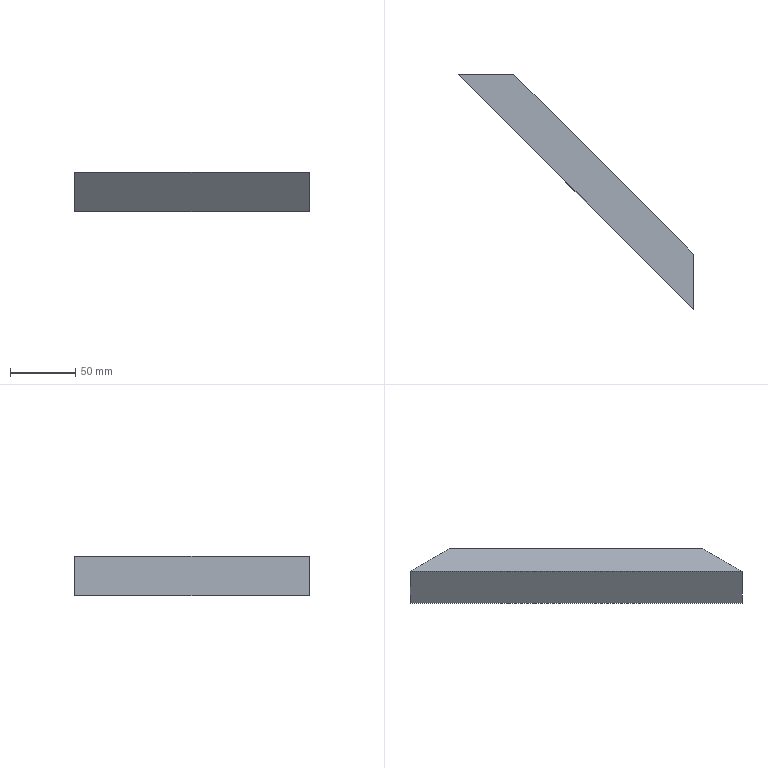Part | NX | features solid 2 | 1 solid | 10 faces | box 180 x 180 x 30 mm | volume 50301 mm3 | plane 10
STEP:
#1=CARTESIAN_POINT('',(212.426,-330.,-60.));
#2=VERTEX_POINT('',#1);
#3=CARTESIAN_POINT('',(170.,-330.,-60.));
#4=VERTEX_POINT('',#3);
#5=CARTESIAN_POINT('',(320.,-330.,-60.));
#6=DIRECTION('',(-1.,0.,0.));
#7=VECTOR('',#6,1000.);
#8=LINE('',#5,#7);
#9=EDGE_CURVE('',#2,#4,#8,.T.);
#10=ORIENTED_EDGE('',*,*,#9,.T.);
#11=CARTESIAN_POINT('',(170.,-330.,-30.));
#12=VERTEX_POINT('',#11);
#13=CARTESIAN_POINT('',(170.,-330.,-30.));
#14=DIRECTION('',(0.,0.,-1.));
#15=VECTOR('',#14,1000.);
#16=LINE('',#13,#15);
#17=EDGE_CURVE('',#12,#4,#16,.T.);
#18=ORIENTED_EDGE('',*,*,#17,.F.);
#19=CARTESIAN_POINT('',(212.426,-330.,-30.));
#20=VERTEX_POINT('',#19);
#21=CARTESIAN_POINT('',(320.,-330.,-30.));
#22=DIRECTION('',(-1.,0.,0.));
#23=VECTOR('',#22,1000.);
#24=LINE('',#21,#23);
#25=EDGE_CURVE('',#20,#12,#24,.T.);
#26=ORIENTED_EDGE('',*,*,#25,.F.);
#27=CARTESIAN_POINT('',(212.426,-330.,-30.));
#28=DIRECTION('',(0.,0.,-1.));
#29=VECTOR('',#28,1000.);
#30=LINE('',#27,#29);
#31=EDGE_CURVE('',#20,#2,#30,.T.);
#32=ORIENTED_EDGE('',*,*,#31,.T.);
#33=EDGE_LOOP('',(#10,#18,#26,#32));
#34=FACE_BOUND('',#33,.T.);
#35=CARTESIAN_POINT('',(209.598,-330.,-32.));
#36=VERTEX_POINT('',#35);
#37=CARTESIAN_POINT('',(209.598,-330.,-58.));
#38=VERTEX_POINT('',#37);
#39=CARTESIAN_POINT('',(209.598,-330.,-30.));
#40=DIRECTION('',(0.,0.,-1.));
#41=VECTOR('',#40,1000.);
#42=LINE('',#39,#41);
#43=EDGE_CURVE('',#36,#38,#42,.T.);
#44=ORIENTED_EDGE('',*,*,#43,.F.);
#45=CARTESIAN_POINT('',(172.828,-330.,-32.));
#46=VERTEX_POINT('',#45);
#47=CARTESIAN_POINT('',(320.,-330.,-32.));
#48=DIRECTION('',(-1.,0.,0.));
#49=VECTOR('',#48,1000.);
#50=LINE('',#47,#49);
#51=EDGE_CURVE('',#36,#46,#50,.T.);
#52=ORIENTED_EDGE('',*,*,#51,.T.);
#53=CARTESIAN_POINT('',(172.828,-330.,-58.));
#54=VERTEX_POINT('',#53);
#55=CARTESIAN_POINT('',(172.828,-330.,-30.));
#56=DIRECTION('',(0.,0.,-1.));
#57=VECTOR('',#56,1000.);
#58=LINE('',#55,#57);
#59=EDGE_CURVE('',#46,#54,#58,.T.);
#60=ORIENTED_EDGE('',*,*,#59,.T.);
#61=CARTESIAN_POINT('',(320.,-330.,-58.));
#62=DIRECTION('',(-1.,0.,0.));
#63=VECTOR('',#62,1000.);
#64=LINE('',#61,#63);
#65=EDGE_CURVE('',#38,#54,#64,.T.);
#66=ORIENTED_EDGE('',*,*,#65,.F.);
#67=EDGE_LOOP('',(#44,#52,#60,#66));
#68=FACE_BOUND('',#67,.T.);
#69=CARTESIAN_POINT('',(320.,-330.,-30.));
#70=DIRECTION('',(0.,1.,0.));
#71=DIRECTION('',(0.,0.,1.));
#72=AXIS2_PLACEMENT_3D('',#69,#70,#71);
#73=PLANE('',#72);
#74=ADVANCED_FACE('',(#34,#68),#73,.T.);
#75=CARTESIAN_POINT('',(350.,-510.,-60.));
#76=VERTEX_POINT('',#75);
#77=CARTESIAN_POINT('',(350.,-467.574,-60.));
#78=VERTEX_POINT('',#77);
#79=CARTESIAN_POINT('',(350.,-402.5,-60.));
#80=DIRECTION('',(0.,1.,0.));
#81=VECTOR('',#80,1000.);
#82=LINE('',#79,#81);
#83=EDGE_CURVE('',#76,#78,#82,.T.);
#84=ORIENTED_EDGE('',*,*,#83,.T.);
#85=CARTESIAN_POINT('',(350.,-467.574,-30.));
#86=VERTEX_POINT('',#85);
#87=CARTESIAN_POINT('',(350.,-467.574,-30.));
#88=DIRECTION('',(0.,0.,-1.));
#89=VECTOR('',#88,1000.);
#90=LINE('',#87,#89);
#91=EDGE_CURVE('',#86,#78,#90,.T.);
#92=ORIENTED_EDGE('',*,*,#91,.F.);
#93=CARTESIAN_POINT('',(350.,-510.,-30.));
#94=VERTEX_POINT('',#93);
#95=CARTESIAN_POINT('',(350.,-402.5,-30.));
#96=DIRECTION('',(0.,1.,0.));
#97=VECTOR('',#96,1000.);
#98=LINE('',#95,#97);
#99=EDGE_CURVE('',#94,#86,#98,.T.);
#100=ORIENTED_EDGE('',*,*,#99,.F.);
#101=CARTESIAN_POINT('',(350.,-510.,-30.));
#102=DIRECTION('',(0.,0.,-1.));
#103=VECTOR('',#102,1000.);
#104=LINE('',#101,#103);
#105=EDGE_CURVE('',#94,#76,#104,.T.);
#106=ORIENTED_EDGE('',*,*,#105,.T.);
#107=EDGE_LOOP('',(#84,#92,#100,#106));
#108=FACE_BOUND('',#107,.T.);
#109=CARTESIAN_POINT('',(350.,-507.172,-32.));
#110=VERTEX_POINT('',#109);
#111=CARTESIAN_POINT('',(350.,-507.172,-58.));
#112=VERTEX_POINT('',#111);
#113=CARTESIAN_POINT('',(350.,-507.172,-30.));
#114=DIRECTION('',(0.,0.,-1.));
#115=VECTOR('',#114,1000.);
#116=LINE('',#113,#115);
#117=EDGE_CURVE('',#110,#112,#116,.T.);
#118=ORIENTED_EDGE('',*,*,#117,.F.);
#119=CARTESIAN_POINT('',(350.,-470.402,-32.));
#120=VERTEX_POINT('',#119);
#121=CARTESIAN_POINT('',(350.,-402.5,-32.));
#122=DIRECTION('',(0.,1.,0.));
#123=VECTOR('',#122,1000.);
#124=LINE('',#121,#123);
#125=EDGE_CURVE('',#110,#120,#124,.T.);
#126=ORIENTED_EDGE('',*,*,#125,.T.);
#127=CARTESIAN_POINT('',(350.,-470.402,-58.));
#128=VERTEX_POINT('',#127);
#129=CARTESIAN_POINT('',(350.,-470.402,-30.));
#130=DIRECTION('',(0.,0.,-1.));
#131=VECTOR('',#130,1000.);
#132=LINE('',#129,#131);
#133=EDGE_CURVE('',#120,#128,#132,.T.);
#134=ORIENTED_EDGE('',*,*,#133,.T.);
#135=CARTESIAN_POINT('',(350.,-402.5,-58.));
#136=DIRECTION('',(0.,1.,0.));
#137=VECTOR('',#136,1000.);
#138=LINE('',#135,#137);
#139=EDGE_CURVE('',#112,#128,#138,.T.);
#140=ORIENTED_EDGE('',*,*,#139,.F.);
#141=EDGE_LOOP('',(#118,#126,#134,#140));
#142=FACE_BOUND('',#141,.T.);
#143=CARTESIAN_POINT('',(350.,-620.,-30.));
#144=DIRECTION('',(1.,0.,0.));
#145=DIRECTION('',(0.,0.,1.));
#146=AXIS2_PLACEMENT_3D('',#143,#144,#145);
#147=PLANE('',#146);
#148=ADVANCED_FACE('',(#108,#142),#147,.T.);
#149=CARTESIAN_POINT('',(212.426,-330.,-60.));
#150=DIRECTION('',(0.7071,-0.7071,0.));
#151=VECTOR('',#150,1000.);
#152=LINE('',#149,#151);
#153=EDGE_CURVE('',#2,#78,#152,.T.);
#154=ORIENTED_EDGE('',*,*,#153,.F.);
#155=ORIENTED_EDGE('',*,*,#31,.F.);
#156=CARTESIAN_POINT('',(212.426,-330.,-30.));
#157=DIRECTION('',(0.7071,-0.7071,0.));
#158=VECTOR('',#157,1000.);
#159=LINE('',#156,#158);
#160=EDGE_CURVE('',#20,#86,#159,.T.);
#161=ORIENTED_EDGE('',*,*,#160,.T.);
#162=ORIENTED_EDGE('',*,*,#91,.T.);
#163=EDGE_LOOP('',(#154,#155,#161,#162));
#164=FACE_BOUND('',#163,.T.);
#165=CARTESIAN_POINT('',(212.426,-330.,-30.));
#166=DIRECTION('',(-0.7071,-0.7071,0.));
#167=DIRECTION('',(-0.7071,0.7071,0.));
#168=AXIS2_PLACEMENT_3D('',#165,#166,#167);
#169=PLANE('',#168);
#170=ADVANCED_FACE('',(#164),#169,.F.);
#171=CARTESIAN_POINT('',(170.,-330.,-60.));
#172=DIRECTION('',(0.7071,-0.7071,0.));
#173=VECTOR('',#172,1000.);
#174=LINE('',#171,#173);
#175=EDGE_CURVE('',#4,#76,#174,.T.);
#176=ORIENTED_EDGE('',*,*,#175,.T.);
#177=ORIENTED_EDGE('',*,*,#105,.F.);
#178=CARTESIAN_POINT('',(170.,-330.,-30.));
#179=DIRECTION('',(0.7071,-0.7071,0.));
#180=VECTOR('',#179,1000.);
#181=LINE('',#178,#180);
#182=EDGE_CURVE('',#12,#94,#181,.T.);
#183=ORIENTED_EDGE('',*,*,#182,.F.);
#184=ORIENTED_EDGE('',*,*,#17,.T.);
#185=EDGE_LOOP('',(#176,#177,#183,#184));
#186=FACE_BOUND('',#185,.T.);
#187=CARTESIAN_POINT('',(170.,-330.,-30.));
#188=DIRECTION('',(-0.7071,-0.7071,0.));
#189=DIRECTION('',(-0.7071,0.7071,0.));
#190=AXIS2_PLACEMENT_3D('',#187,#188,#189);
#191=PLANE('',#190);
#192=ADVANCED_FACE('',(#186),#191,.T.);
#193=ORIENTED_EDGE('',*,*,#25,.T.);
#194=ORIENTED_EDGE('',*,*,#182,.T.);
#195=ORIENTED_EDGE('',*,*,#99,.T.);
#196=ORIENTED_EDGE('',*,*,#160,.F.);
#197=EDGE_LOOP('',(#193,#194,#195,#196));
#198=FACE_BOUND('',#197,.T.);
#199=CARTESIAN_POINT('',(255.607,-402.5,-30.));
#200=DIRECTION('',(0.,0.,1.));
#201=DIRECTION('',(-1.,0.,0.));
#202=AXIS2_PLACEMENT_3D('',#199,#200,#201);
#203=PLANE('',#202);
#204=ADVANCED_FACE('',(#198),#203,.T.);
#205=ORIENTED_EDGE('',*,*,#9,.F.);
#206=ORIENTED_EDGE('',*,*,#153,.T.);
#207=ORIENTED_EDGE('',*,*,#83,.F.);
#208=ORIENTED_EDGE('',*,*,#175,.F.);
#209=EDGE_LOOP('',(#205,#206,#207,#208));
#210=FACE_BOUND('',#209,.T.);
#211=CARTESIAN_POINT('',(255.607,-402.5,-60.));
#212=DIRECTION('',(0.,0.,1.));
#213=DIRECTION('',(-1.,0.,0.));
#214=AXIS2_PLACEMENT_3D('',#211,#212,#213);
#215=PLANE('',#214);
#216=ADVANCED_FACE('',(#210),#215,.F.);
#217=CARTESIAN_POINT('',(211.012,-331.414,-58.));
#218=DIRECTION('',(0.7071,-0.7071,0.));
#219=VECTOR('',#218,1000.);
#220=LINE('',#217,#219);
#221=EDGE_CURVE('',#38,#128,#220,.T.);
#222=ORIENTED_EDGE('',*,*,#221,.T.);
#223=ORIENTED_EDGE('',*,*,#133,.F.);
#224=CARTESIAN_POINT('',(211.012,-331.414,-32.));
#225=DIRECTION('',(0.7071,-0.7071,0.));
#226=VECTOR('',#225,1000.);
#227=LINE('',#224,#226);
#228=EDGE_CURVE('',#36,#120,#227,.T.);
#229=ORIENTED_EDGE('',*,*,#228,.F.);
#230=ORIENTED_EDGE('',*,*,#43,.T.);
#231=EDGE_LOOP('',(#222,#223,#229,#230));
#232=FACE_BOUND('',#231,.T.);
#233=CARTESIAN_POINT('',(211.012,-331.414,-30.));
#234=DIRECTION('',(-0.7071,-0.7071,0.));
#235=DIRECTION('',(-0.7071,0.7071,0.));
#236=AXIS2_PLACEMENT_3D('',#233,#234,#235);
#237=PLANE('',#236);
#238=ADVANCED_FACE('',(#232),#237,.T.);
#239=CARTESIAN_POINT('',(171.414,-328.586,-58.));
#240=DIRECTION('',(0.7071,-0.7071,0.));
#241=VECTOR('',#240,1000.);
#242=LINE('',#239,#241);
#243=EDGE_CURVE('',#54,#112,#242,.T.);
#244=ORIENTED_EDGE('',*,*,#243,.F.);
#245=ORIENTED_EDGE('',*,*,#59,.F.);
#246=CARTESIAN_POINT('',(171.414,-328.586,-32.));
#247=DIRECTION('',(0.7071,-0.7071,0.));
#248=VECTOR('',#247,1000.);
#249=LINE('',#246,#248);
#250=EDGE_CURVE('',#46,#110,#249,.T.);
#251=ORIENTED_EDGE('',*,*,#250,.T.);
#252=ORIENTED_EDGE('',*,*,#117,.T.);
#253=EDGE_LOOP('',(#244,#245,#251,#252));
#254=FACE_BOUND('',#253,.T.);
#255=CARTESIAN_POINT('',(171.414,-328.586,-30.));
#256=DIRECTION('',(-0.7071,-0.7071,0.));
#257=DIRECTION('',(-0.7071,0.7071,0.));
#258=AXIS2_PLACEMENT_3D('',#255,#256,#257);
#259=PLANE('',#258);
#260=ADVANCED_FACE('',(#254),#259,.F.);
#261=ORIENTED_EDGE('',*,*,#51,.F.);
#262=ORIENTED_EDGE('',*,*,#228,.T.);
#263=ORIENTED_EDGE('',*,*,#125,.F.);
#264=ORIENTED_EDGE('',*,*,#250,.F.);
#265=EDGE_LOOP('',(#261,#262,#263,#264));
#266=FACE_BOUND('',#265,.T.);
#267=CARTESIAN_POINT('',(255.607,-402.5,-32.));
#268=DIRECTION('',(0.,0.,1.));
#269=DIRECTION('',(-1.,0.,0.));
#270=AXIS2_PLACEMENT_3D('',#267,#268,#269);
#271=PLANE('',#270);
#272=ADVANCED_FACE('',(#266),#271,.F.);
#273=ORIENTED_EDGE('',*,*,#65,.T.);
#274=ORIENTED_EDGE('',*,*,#243,.T.);
#275=ORIENTED_EDGE('',*,*,#139,.T.);
#276=ORIENTED_EDGE('',*,*,#221,.F.);
#277=EDGE_LOOP('',(#273,#274,#275,#276));
#278=FACE_BOUND('',#277,.T.);
#279=CARTESIAN_POINT('',(255.607,-402.5,-58.));
#280=DIRECTION('',(0.,0.,1.));
#281=DIRECTION('',(-1.,0.,0.));
#282=AXIS2_PLACEMENT_3D('',#279,#280,#281);
#283=PLANE('',#282);
#284=ADVANCED_FACE('',(#278),#283,.T.);
#285=CLOSED_SHELL('',(#74,#148,#170,#192,#204,#216,#238,#260,#272,#284));
#286=MANIFOLD_SOLID_BREP('',#285);
#287=(LENGTH_UNIT()NAMED_UNIT(*)SI_UNIT(.MILLI.,.METRE.));
#288=UNCERTAINTY_MEASURE_WITH_UNIT(LENGTH_MEASURE(0.00001),#287,'','');
#289=(NAMED_UNIT(*)PLANE_ANGLE_UNIT()SI_UNIT($,.RADIAN.));
#290=(NAMED_UNIT(*)SI_UNIT($,.STERADIAN.)SOLID_ANGLE_UNIT());
#291=(GEOMETRIC_REPRESENTATION_CONTEXT(3)GLOBAL_UNCERTAINTY_ASSIGNED_CONTEXT((#288))GLOBAL_UNIT_ASSIGNED_CONTEXT((#287,#289,#290))REPRESENTATION_CONTEXT('',''));
#292=ADVANCED_BREP_SHAPE_REPRESENTATION('',(#286),#291);